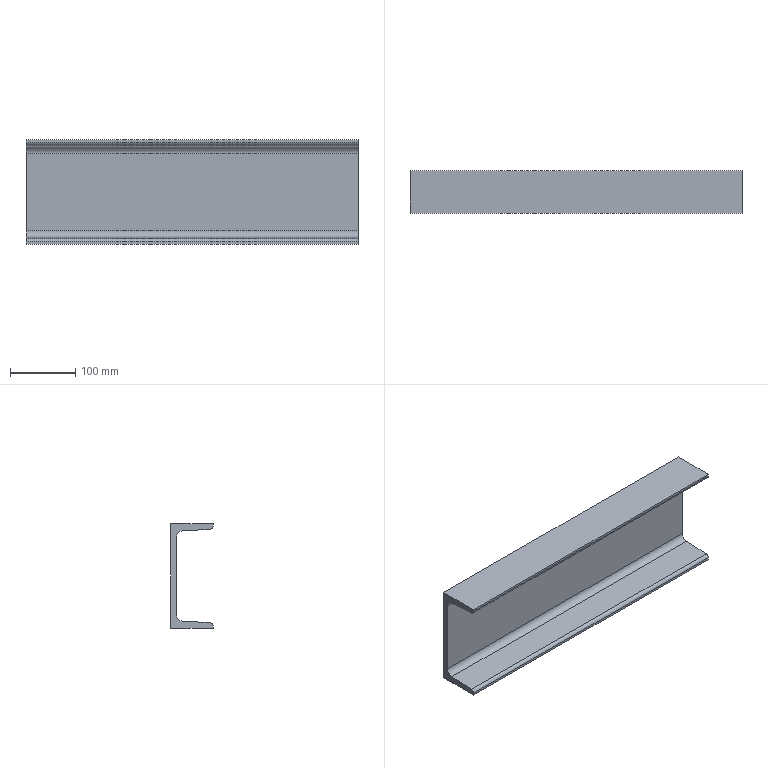Part | STEP file | 07-Channel 100x48_default<machining> | 1 solid | 14 faces | box 509 x 65 x 160 mm | volume 1267662 mm3 | plane 10 | cylinder 4 | commonest cylinder face diameters 10 x2 20 x2
STEP:
#1=CARTESIAN_POINT('',(0.,0.,0.));
#2=DIRECTION('',(0.,0.,1.));
#3=DIRECTION('',(1.,0.,0.));
#4=AXIS2_PLACEMENT_3D('',#1,#2,#3);
#5=CARTESIAN_POINT('',(0.,-65.,-160.));
#6=VERTEX_POINT('',#5);
#7=CARTESIAN_POINT('',(0.,0.,-160.));
#8=VERTEX_POINT('',#7);
#9=CARTESIAN_POINT('',(0.,0.,-160.));
#10=DIRECTION('',(0.,1.,0.));
#11=VECTOR('',#10,1.);
#12=LINE('',#9,#11);
#13=CARTESIAN_POINT('',(509.,0.,-160.));
#14=DIRECTION('',(0.,0.,1.));
#15=DIRECTION('',(1.,0.,0.));
#16=AXIS2_PLACEMENT_3D('',#13,#14,#15);
#17=PLANE('',#16);
#18=CARTESIAN_POINT('',(-509.,0.));
#19=DIRECTION('',(0.,1.));
#20=VECTOR('',#19,1.);
#21=LINE('',#18,#20);
#22=(GEOMETRIC_REPRESENTATION_CONTEXT(2)PARAMETRIC_REPRESENTATION_CONTEXT()REPRESENTATION_CONTEXT('',''));
#23=DEFINITIONAL_REPRESENTATION('',(#21),#22);
#24=PCURVE('',#17,#23);
#25=CARTESIAN_POINT('',(0.,-60.,-156.59));
#26=DIRECTION('',(1.,0.,0.));
#27=DIRECTION('',(0.,0.,-1.));
#28=AXIS2_PLACEMENT_3D('',#25,#26,#27);
#29=PLANE('',#28);
#30=CARTESIAN_POINT('',(3.41,60.));
#31=DIRECTION('',(0.,1.));
#32=VECTOR('',#31,1.);
#33=LINE('',#30,#32);
#34=(GEOMETRIC_REPRESENTATION_CONTEXT(2)PARAMETRIC_REPRESENTATION_CONTEXT()REPRESENTATION_CONTEXT('',''));
#35=DEFINITIONAL_REPRESENTATION('',(#33),#34);
#36=PCURVE('',#29,#35);
#37=SURFACE_CURVE('',#12,(#24,#36),.PCURVE_S1.);
#38=EDGE_CURVE('',#6,#8,#37,.T.);
#39=ORIENTED_EDGE('',*,*,#38,.T.);
#40=CARTESIAN_POINT('',(509.,0.,-160.));
#41=VERTEX_POINT('',#40);
#42=CARTESIAN_POINT('',(509.,0.,-160.));
#43=DIRECTION('',(-1.,0.,0.));
#44=VECTOR('',#43,1.);
#45=LINE('',#42,#44);
#46=CARTESIAN_POINT('',(0.,0.));
#47=DIRECTION('',(-1.,0.));
#48=VECTOR('',#47,1.);
#49=LINE('',#46,#48);
#50=(GEOMETRIC_REPRESENTATION_CONTEXT(2)PARAMETRIC_REPRESENTATION_CONTEXT()REPRESENTATION_CONTEXT('',''));
#51=DEFINITIONAL_REPRESENTATION('',(#49),#50);
#52=PCURVE('',#17,#51);
#53=CARTESIAN_POINT('',(509.,0.,0.));
#54=DIRECTION('',(0.,-1.,0.));
#55=DIRECTION('',(0.,0.,-1.));
#56=AXIS2_PLACEMENT_3D('',#53,#54,#55);
#57=PLANE('',#56);
#58=CARTESIAN_POINT('',(160.,0.));
#59=DIRECTION('',(0.,-1.));
#60=VECTOR('',#59,1.);
#61=LINE('',#58,#60);
#62=(GEOMETRIC_REPRESENTATION_CONTEXT(2)PARAMETRIC_REPRESENTATION_CONTEXT()REPRESENTATION_CONTEXT('',''));
#63=DEFINITIONAL_REPRESENTATION('',(#61),#62);
#64=PCURVE('',#57,#63);
#65=SURFACE_CURVE('',#45,(#52,#64),.PCURVE_S1.);
#66=EDGE_CURVE('',#41,#8,#65,.T.);
#67=ORIENTED_EDGE('',*,*,#66,.F.);
#68=CARTESIAN_POINT('',(509.,-65.,-160.));
#69=VERTEX_POINT('',#68);
#70=CARTESIAN_POINT('',(509.,0.,-160.));
#71=DIRECTION('',(0.,1.,0.));
#72=VECTOR('',#71,1.);
#73=LINE('',#70,#72);
#74=CARTESIAN_POINT('',(0.,0.));
#75=DIRECTION('',(0.,1.));
#76=VECTOR('',#75,1.);
#77=LINE('',#74,#76);
#78=(GEOMETRIC_REPRESENTATION_CONTEXT(2)PARAMETRIC_REPRESENTATION_CONTEXT()REPRESENTATION_CONTEXT('',''));
#79=DEFINITIONAL_REPRESENTATION('',(#77),#78);
#80=PCURVE('',#17,#79);
#81=CARTESIAN_POINT('',(509.,-60.,-156.59));
#82=DIRECTION('',(1.,0.,0.));
#83=DIRECTION('',(0.,0.,-1.));
#84=AXIS2_PLACEMENT_3D('',#81,#82,#83);
#85=PLANE('',#84);
#86=CARTESIAN_POINT('',(3.41,60.));
#87=DIRECTION('',(0.,1.));
#88=VECTOR('',#87,1.);
#89=LINE('',#86,#88);
#90=(GEOMETRIC_REPRESENTATION_CONTEXT(2)PARAMETRIC_REPRESENTATION_CONTEXT()REPRESENTATION_CONTEXT('',''));
#91=DEFINITIONAL_REPRESENTATION('',(#89),#90);
#92=PCURVE('',#85,#91);
#93=SURFACE_CURVE('',#73,(#80,#92),.PCURVE_S1.);
#94=EDGE_CURVE('',#69,#41,#93,.T.);
#95=ORIENTED_EDGE('',*,*,#94,.F.);
#96=CARTESIAN_POINT('',(509.,-65.,-160.));
#97=DIRECTION('',(-1.,0.,0.));
#98=VECTOR('',#97,1.);
#99=LINE('',#96,#98);
#100=CARTESIAN_POINT('',(0.,-65.));
#101=DIRECTION('',(-1.,0.));
#102=VECTOR('',#101,1.);
#103=LINE('',#100,#102);
#104=(GEOMETRIC_REPRESENTATION_CONTEXT(2)PARAMETRIC_REPRESENTATION_CONTEXT()REPRESENTATION_CONTEXT('',''));
#105=DEFINITIONAL_REPRESENTATION('',(#103),#104);
#106=PCURVE('',#17,#105);
#107=CARTESIAN_POINT('',(509.,-65.,-156.59));
#108=DIRECTION('',(0.,1.,0.));
#109=DIRECTION('',(0.,0.,1.));
#110=AXIS2_PLACEMENT_3D('',#107,#108,#109);
#111=PLANE('',#110);
#112=CARTESIAN_POINT('',(-3.41,0.));
#113=DIRECTION('',(0.,-1.));
#114=VECTOR('',#113,1.);
#115=LINE('',#112,#114);
#116=(GEOMETRIC_REPRESENTATION_CONTEXT(2)PARAMETRIC_REPRESENTATION_CONTEXT()REPRESENTATION_CONTEXT('',''));
#117=DEFINITIONAL_REPRESENTATION('',(#115),#116);
#118=PCURVE('',#111,#117);
#119=SURFACE_CURVE('',#99,(#106,#118),.PCURVE_S1.);
#120=EDGE_CURVE('',#69,#6,#119,.T.);
#121=ORIENTED_EDGE('',*,*,#120,.T.);
#122=EDGE_LOOP('',(#39,#67,#95,#121));
#123=FACE_BOUND('',#122,.T.);
#124=ADVANCED_FACE('',(#123),#17,.F.);
#125=CARTESIAN_POINT('',(0.,0.,0.));
#126=VERTEX_POINT('',#125);
#127=CARTESIAN_POINT('',(0.,0.,0.));
#128=DIRECTION('',(0.,0.,1.));
#129=VECTOR('',#128,1.);
#130=LINE('',#127,#129);
#131=CARTESIAN_POINT('',(0.,-509.));
#132=DIRECTION('',(-1.,0.));
#133=VECTOR('',#132,1.);
#134=LINE('',#131,#133);
#135=(GEOMETRIC_REPRESENTATION_CONTEXT(2)PARAMETRIC_REPRESENTATION_CONTEXT()REPRESENTATION_CONTEXT('',''));
#136=DEFINITIONAL_REPRESENTATION('',(#134),#135);
#137=PCURVE('',#57,#136);
#138=CARTESIAN_POINT('',(-156.59,60.));
#139=DIRECTION('',(-1.,0.));
#140=VECTOR('',#139,1.);
#141=LINE('',#138,#140);
#142=(GEOMETRIC_REPRESENTATION_CONTEXT(2)PARAMETRIC_REPRESENTATION_CONTEXT()REPRESENTATION_CONTEXT('',''));
#143=DEFINITIONAL_REPRESENTATION('',(#141),#142);
#144=PCURVE('',#29,#143);
#145=SURFACE_CURVE('',#130,(#137,#144),.PCURVE_S1.);
#146=EDGE_CURVE('',#8,#126,#145,.T.);
#147=ORIENTED_EDGE('',*,*,#146,.T.);
#148=CARTESIAN_POINT('',(509.,0.,0.));
#149=VERTEX_POINT('',#148);
#150=CARTESIAN_POINT('',(509.,0.,0.));
#151=DIRECTION('',(-1.,0.,0.));
#152=VECTOR('',#151,1.);
#153=LINE('',#150,#152);
#154=CARTESIAN_POINT('',(0.,0.));
#155=DIRECTION('',(0.,-1.));
#156=VECTOR('',#155,1.);
#157=LINE('',#154,#156);
#158=(GEOMETRIC_REPRESENTATION_CONTEXT(2)PARAMETRIC_REPRESENTATION_CONTEXT()REPRESENTATION_CONTEXT('',''));
#159=DEFINITIONAL_REPRESENTATION('',(#157),#158);
#160=PCURVE('',#57,#159);
#161=CARTESIAN_POINT('',(509.,0.,0.));
#162=DIRECTION('',(0.,0.,-1.));
#163=DIRECTION('',(0.,1.,0.));
#164=AXIS2_PLACEMENT_3D('',#161,#162,#163);
#165=PLANE('',#164);
#166=CARTESIAN_POINT('',(0.,0.));
#167=DIRECTION('',(0.,-1.));
#168=VECTOR('',#167,1.);
#169=LINE('',#166,#168);
#170=(GEOMETRIC_REPRESENTATION_CONTEXT(2)PARAMETRIC_REPRESENTATION_CONTEXT()REPRESENTATION_CONTEXT('',''));
#171=DEFINITIONAL_REPRESENTATION('',(#169),#170);
#172=PCURVE('',#165,#171);
#173=SURFACE_CURVE('',#153,(#160,#172),.PCURVE_S1.);
#174=EDGE_CURVE('',#149,#126,#173,.T.);
#175=ORIENTED_EDGE('',*,*,#174,.F.);
#176=CARTESIAN_POINT('',(509.,0.,0.));
#177=DIRECTION('',(0.,0.,1.));
#178=VECTOR('',#177,1.);
#179=LINE('',#176,#178);
#180=CARTESIAN_POINT('',(0.,0.));
#181=DIRECTION('',(-1.,0.));
#182=VECTOR('',#181,1.);
#183=LINE('',#180,#182);
#184=(GEOMETRIC_REPRESENTATION_CONTEXT(2)PARAMETRIC_REPRESENTATION_CONTEXT()REPRESENTATION_CONTEXT('',''));
#185=DEFINITIONAL_REPRESENTATION('',(#183),#184);
#186=PCURVE('',#57,#185);
#187=CARTESIAN_POINT('',(-156.59,60.));
#188=DIRECTION('',(-1.,0.));
#189=VECTOR('',#188,1.);
#190=LINE('',#187,#189);
#191=(GEOMETRIC_REPRESENTATION_CONTEXT(2)PARAMETRIC_REPRESENTATION_CONTEXT()REPRESENTATION_CONTEXT('',''));
#192=DEFINITIONAL_REPRESENTATION('',(#190),#191);
#193=PCURVE('',#85,#192);
#194=SURFACE_CURVE('',#179,(#186,#193),.PCURVE_S1.);
#195=EDGE_CURVE('',#41,#149,#194,.T.);
#196=ORIENTED_EDGE('',*,*,#195,.F.);
#197=ORIENTED_EDGE('',*,*,#66,.T.);
#198=EDGE_LOOP('',(#147,#175,#196,#197));
#199=FACE_BOUND('',#198,.T.);
#200=ADVANCED_FACE('',(#199),#57,.F.);
#201=CARTESIAN_POINT('',(0.,-65.,0.));
#202=VERTEX_POINT('',#201);
#203=CARTESIAN_POINT('',(0.,0.,0.));
#204=DIRECTION('',(0.,-1.,0.));
#205=VECTOR('',#204,1.);
#206=LINE('',#203,#205);
#207=CARTESIAN_POINT('',(0.,-509.));
#208=DIRECTION('',(-1.,0.));
#209=VECTOR('',#208,1.);
#210=LINE('',#207,#209);
#211=(GEOMETRIC_REPRESENTATION_CONTEXT(2)PARAMETRIC_REPRESENTATION_CONTEXT()REPRESENTATION_CONTEXT('',''));
#212=DEFINITIONAL_REPRESENTATION('',(#210),#211);
#213=PCURVE('',#165,#212);
#214=CARTESIAN_POINT('',(-156.59,60.));
#215=DIRECTION('',(0.,-1.));
#216=VECTOR('',#215,1.);
#217=LINE('',#214,#216);
#218=(GEOMETRIC_REPRESENTATION_CONTEXT(2)PARAMETRIC_REPRESENTATION_CONTEXT()REPRESENTATION_CONTEXT('',''));
#219=DEFINITIONAL_REPRESENTATION('',(#217),#218);
#220=PCURVE('',#29,#219);
#221=SURFACE_CURVE('',#206,(#213,#220),.PCURVE_S1.);
#222=EDGE_CURVE('',#126,#202,#221,.T.);
#223=ORIENTED_EDGE('',*,*,#222,.T.);
#224=CARTESIAN_POINT('',(509.,-65.,0.));
#225=VERTEX_POINT('',#224);
#226=CARTESIAN_POINT('',(509.,-65.,0.));
#227=DIRECTION('',(-1.,0.,0.));
#228=VECTOR('',#227,1.);
#229=LINE('',#226,#228);
#230=CARTESIAN_POINT('',(-65.,0.));
#231=DIRECTION('',(0.,-1.));
#232=VECTOR('',#231,1.);
#233=LINE('',#230,#232);
#234=(GEOMETRIC_REPRESENTATION_CONTEXT(2)PARAMETRIC_REPRESENTATION_CONTEXT()REPRESENTATION_CONTEXT('',''));
#235=DEFINITIONAL_REPRESENTATION('',(#233),#234);
#236=PCURVE('',#165,#235);
#237=CARTESIAN_POINT('',(509.,-65.,-3.41));
#238=DIRECTION('',(0.,1.,0.));
#239=DIRECTION('',(0.,0.,1.));
#240=AXIS2_PLACEMENT_3D('',#237,#238,#239);
#241=PLANE('',#240);
#242=CARTESIAN_POINT('',(3.41,0.));
#243=DIRECTION('',(0.,-1.));
#244=VECTOR('',#243,1.);
#245=LINE('',#242,#244);
#246=(GEOMETRIC_REPRESENTATION_CONTEXT(2)PARAMETRIC_REPRESENTATION_CONTEXT()REPRESENTATION_CONTEXT('',''));
#247=DEFINITIONAL_REPRESENTATION('',(#245),#246);
#248=PCURVE('',#241,#247);
#249=SURFACE_CURVE('',#229,(#236,#248),.PCURVE_S1.);
#250=EDGE_CURVE('',#225,#202,#249,.T.);
#251=ORIENTED_EDGE('',*,*,#250,.F.);
#252=CARTESIAN_POINT('',(509.,0.,0.));
#253=DIRECTION('',(0.,-1.,0.));
#254=VECTOR('',#253,1.);
#255=LINE('',#252,#254);
#256=CARTESIAN_POINT('',(0.,0.));
#257=DIRECTION('',(-1.,0.));
#258=VECTOR('',#257,1.);
#259=LINE('',#256,#258);
#260=(GEOMETRIC_REPRESENTATION_CONTEXT(2)PARAMETRIC_REPRESENTATION_CONTEXT()REPRESENTATION_CONTEXT('',''));
#261=DEFINITIONAL_REPRESENTATION('',(#259),#260);
#262=PCURVE('',#165,#261);
#263=CARTESIAN_POINT('',(-156.59,60.));
#264=DIRECTION('',(0.,-1.));
#265=VECTOR('',#264,1.);
#266=LINE('',#263,#265);
#267=(GEOMETRIC_REPRESENTATION_CONTEXT(2)PARAMETRIC_REPRESENTATION_CONTEXT()REPRESENTATION_CONTEXT('',''));
#268=DEFINITIONAL_REPRESENTATION('',(#266),#267);
#269=PCURVE('',#85,#268);
#270=SURFACE_CURVE('',#255,(#262,#269),.PCURVE_S1.);
#271=EDGE_CURVE('',#149,#225,#270,.T.);
#272=ORIENTED_EDGE('',*,*,#271,.F.);
#273=ORIENTED_EDGE('',*,*,#174,.T.);
#274=EDGE_LOOP('',(#223,#251,#272,#273));
#275=FACE_BOUND('',#274,.T.);
#276=ADVANCED_FACE('',(#275),#165,.F.);
#277=CARTESIAN_POINT('',(0.,-65.,-3.41));
#278=VERTEX_POINT('',#277);
#279=CARTESIAN_POINT('',(0.,-65.,-3.41));
#280=DIRECTION('',(0.,0.,-1.));
#281=VECTOR('',#280,1.);
#282=LINE('',#279,#281);
#283=CARTESIAN_POINT('',(0.,-509.));
#284=DIRECTION('',(-1.,0.));
#285=VECTOR('',#284,1.);
#286=LINE('',#283,#285);
#287=(GEOMETRIC_REPRESENTATION_CONTEXT(2)PARAMETRIC_REPRESENTATION_CONTEXT()REPRESENTATION_CONTEXT('',''));
#288=DEFINITIONAL_REPRESENTATION('',(#286),#287);
#289=PCURVE('',#241,#288);
#290=CARTESIAN_POINT('',(-153.18,-5.));
#291=DIRECTION('',(1.,0.));
#292=VECTOR('',#291,1.);
#293=LINE('',#290,#292);
#294=(GEOMETRIC_REPRESENTATION_CONTEXT(2)PARAMETRIC_REPRESENTATION_CONTEXT()REPRESENTATION_CONTEXT('',''));
#295=DEFINITIONAL_REPRESENTATION('',(#293),#294);
#296=PCURVE('',#29,#295);
#297=SURFACE_CURVE('',#282,(#289,#296),.PCURVE_S1.);
#298=EDGE_CURVE('',#202,#278,#297,.T.);
#299=ORIENTED_EDGE('',*,*,#298,.T.);
#300=CARTESIAN_POINT('',(509.,-65.,-3.41));
#301=VERTEX_POINT('',#300);
#302=CARTESIAN_POINT('',(509.,-65.,-3.41));
#303=DIRECTION('',(-1.,0.,0.));
#304=VECTOR('',#303,1.);
#305=LINE('',#302,#304);
#306=CARTESIAN_POINT('',(0.,0.));
#307=DIRECTION('',(0.,-1.));
#308=VECTOR('',#307,1.);
#309=LINE('',#306,#308);
#310=(GEOMETRIC_REPRESENTATION_CONTEXT(2)PARAMETRIC_REPRESENTATION_CONTEXT()REPRESENTATION_CONTEXT('',''));
#311=DEFINITIONAL_REPRESENTATION('',(#309),#310);
#312=PCURVE('',#241,#311);
#313=CARTESIAN_POINT('',(509.,-60.,-3.41));
#314=DIRECTION('',(-1.,0.,0.));
#315=DIRECTION('',(0.,0.,1.));
#316=AXIS2_PLACEMENT_3D('',#313,#314,#315);
#317=CYLINDRICAL_SURFACE('',#316,5.);
#318=CARTESIAN_POINT('',(4.712,0.));
#319=DIRECTION('',(0.,1.));
#320=VECTOR('',#319,1.);
#321=LINE('',#318,#320);
#322=(GEOMETRIC_REPRESENTATION_CONTEXT(2)PARAMETRIC_REPRESENTATION_CONTEXT()REPRESENTATION_CONTEXT('',''));
#323=DEFINITIONAL_REPRESENTATION('',(#321),#322);
#324=PCURVE('',#317,#323);
#325=SURFACE_CURVE('',#305,(#312,#324),.PCURVE_S1.);
#326=EDGE_CURVE('',#301,#278,#325,.T.);
#327=ORIENTED_EDGE('',*,*,#326,.F.);
#328=CARTESIAN_POINT('',(509.,-65.,-3.41));
#329=DIRECTION('',(0.,0.,-1.));
#330=VECTOR('',#329,1.);
#331=LINE('',#328,#330);
#332=CARTESIAN_POINT('',(0.,0.));
#333=DIRECTION('',(-1.,0.));
#334=VECTOR('',#333,1.);
#335=LINE('',#332,#334);
#336=(GEOMETRIC_REPRESENTATION_CONTEXT(2)PARAMETRIC_REPRESENTATION_CONTEXT()REPRESENTATION_CONTEXT('',''));
#337=DEFINITIONAL_REPRESENTATION('',(#335),#336);
#338=PCURVE('',#241,#337);
#339=CARTESIAN_POINT('',(-153.18,-5.));
#340=DIRECTION('',(1.,0.));
#341=VECTOR('',#340,1.);
#342=LINE('',#339,#341);
#343=(GEOMETRIC_REPRESENTATION_CONTEXT(2)PARAMETRIC_REPRESENTATION_CONTEXT()REPRESENTATION_CONTEXT('',''));
#344=DEFINITIONAL_REPRESENTATION('',(#342),#343);
#345=PCURVE('',#85,#344);
#346=SURFACE_CURVE('',#331,(#338,#345),.PCURVE_S1.);
#347=EDGE_CURVE('',#225,#301,#346,.T.);
#348=ORIENTED_EDGE('',*,*,#347,.F.);
#349=ORIENTED_EDGE('',*,*,#250,.T.);
#350=EDGE_LOOP('',(#299,#327,#348,#349));
#351=FACE_BOUND('',#350,.T.);
#352=ADVANCED_FACE('',(#351),#241,.F.);
#353=CARTESIAN_POINT('',(0.,-60.287,-8.402));
#354=VERTEX_POINT('',#353);
#355=CARTESIAN_POINT('',(0.,-60.,-3.41));
#356=DIRECTION('',(1.,0.,0.));
#357=DIRECTION('',(0.,0.,-1.));
#358=AXIS2_PLACEMENT_3D('',#355,#356,#357);
#359=CIRCLE('',#358,5.);
#360=CARTESIAN_POINT('',(9.425,509.));
#361=DIRECTION('',(-1.,0.));
#362=VECTOR('',#361,1.);
#363=LINE('',#360,#362);
#364=(GEOMETRIC_REPRESENTATION_CONTEXT(2)PARAMETRIC_REPRESENTATION_CONTEXT()REPRESENTATION_CONTEXT('',''));
#365=DEFINITIONAL_REPRESENTATION('',(#363),#364);
#366=PCURVE('',#317,#365);
#367=CARTESIAN_POINT('',(-153.18,0.));
#368=DIRECTION('',(1.,0.));
#369=AXIS2_PLACEMENT_2D('',#367,#368);
#370=CIRCLE('',#369,5.);
#371=(GEOMETRIC_REPRESENTATION_CONTEXT(2)PARAMETRIC_REPRESENTATION_CONTEXT()REPRESENTATION_CONTEXT('',''));
#372=DEFINITIONAL_REPRESENTATION('',(#370),#371);
#373=PCURVE('',#29,#372);
#374=SURFACE_CURVE('',#359,(#366,#373),.PCURVE_S1.);
#375=EDGE_CURVE('',#278,#354,#374,.T.);
#376=ORIENTED_EDGE('',*,*,#375,.T.);
#377=CARTESIAN_POINT('',(509.,-60.287,-8.402));
#378=VERTEX_POINT('',#377);
#379=CARTESIAN_POINT('',(509.,-60.287,-8.402));
#380=DIRECTION('',(-1.,0.,0.));
#381=VECTOR('',#380,1.);
#382=LINE('',#379,#381);
#383=CARTESIAN_POINT('',(3.199,0.));
#384=DIRECTION('',(0.,1.));
#385=VECTOR('',#384,1.);
#386=LINE('',#383,#385);
#387=(GEOMETRIC_REPRESENTATION_CONTEXT(2)PARAMETRIC_REPRESENTATION_CONTEXT()REPRESENTATION_CONTEXT('',''));
#388=DEFINITIONAL_REPRESENTATION('',(#386),#387);
#389=PCURVE('',#317,#388);
#390=CARTESIAN_POINT('',(509.,-17.926,-10.838));
#391=DIRECTION('',(0.,0.05743,0.9983));
#392=DIRECTION('',(0.,-0.9983,0.05743));
#393=AXIS2_PLACEMENT_3D('',#390,#391,#392);
#394=PLANE('',#393);
#395=CARTESIAN_POINT('',(42.431,0.));
#396=DIRECTION('',(0.,-1.));
#397=VECTOR('',#396,1.);
#398=LINE('',#395,#397);
#399=(GEOMETRIC_REPRESENTATION_CONTEXT(2)PARAMETRIC_REPRESENTATION_CONTEXT()REPRESENTATION_CONTEXT('',''));
#400=DEFINITIONAL_REPRESENTATION('',(#398),#399);
#401=PCURVE('',#394,#400);
#402=SURFACE_CURVE('',#382,(#389,#401),.PCURVE_S1.);
#403=EDGE_CURVE('',#378,#354,#402,.T.);
#404=ORIENTED_EDGE('',*,*,#403,.F.);
#405=CARTESIAN_POINT('',(509.,-60.,-3.41));
#406=DIRECTION('',(1.,0.,0.));
#407=DIRECTION('',(0.,0.,-1.));
#408=AXIS2_PLACEMENT_3D('',#405,#406,#407);
#409=CIRCLE('',#408,5.);
#410=CARTESIAN_POINT('',(9.425,0.));
#411=DIRECTION('',(-1.,0.));
#412=VECTOR('',#411,1.);
#413=LINE('',#410,#412);
#414=(GEOMETRIC_REPRESENTATION_CONTEXT(2)PARAMETRIC_REPRESENTATION_CONTEXT()REPRESENTATION_CONTEXT('',''));
#415=DEFINITIONAL_REPRESENTATION('',(#413),#414);
#416=PCURVE('',#317,#415);
#417=CARTESIAN_POINT('',(-153.18,0.));
#418=DIRECTION('',(1.,0.));
#419=AXIS2_PLACEMENT_2D('',#417,#418);
#420=CIRCLE('',#419,5.);
#421=(GEOMETRIC_REPRESENTATION_CONTEXT(2)PARAMETRIC_REPRESENTATION_CONTEXT()REPRESENTATION_CONTEXT('',''));
#422=DEFINITIONAL_REPRESENTATION('',(#420),#421);
#423=PCURVE('',#85,#422);
#424=SURFACE_CURVE('',#409,(#416,#423),.PCURVE_S1.);
#425=EDGE_CURVE('',#301,#378,#424,.T.);
#426=ORIENTED_EDGE('',*,*,#425,.F.);
#427=ORIENTED_EDGE('',*,*,#326,.T.);
#428=EDGE_LOOP('',(#376,#404,#426,#427));
#429=FACE_BOUND('',#428,.T.);
#430=ADVANCED_FACE('',(#429),#317,.T.);
#431=CARTESIAN_POINT('',(0.,-17.926,-10.838));
#432=VERTEX_POINT('',#431);
#433=CARTESIAN_POINT('',(0.,-17.926,-10.838));
#434=DIRECTION('',(0.,0.9983,-0.05743));
#435=VECTOR('',#434,1.);
#436=LINE('',#433,#435);
#437=CARTESIAN_POINT('',(0.,-509.));
#438=DIRECTION('',(-1.,0.));
#439=VECTOR('',#438,1.);
#440=LINE('',#437,#439);
#441=(GEOMETRIC_REPRESENTATION_CONTEXT(2)PARAMETRIC_REPRESENTATION_CONTEXT()REPRESENTATION_CONTEXT('',''));
#442=DEFINITIONAL_REPRESENTATION('',(#440),#441);
#443=PCURVE('',#394,#442);
#444=CARTESIAN_POINT('',(-145.752,42.074));
#445=DIRECTION('',(0.05743,0.9983));
#446=VECTOR('',#445,1.);
#447=LINE('',#444,#446);
#448=(GEOMETRIC_REPRESENTATION_CONTEXT(2)PARAMETRIC_REPRESENTATION_CONTEXT()REPRESENTATION_CONTEXT('',''));
#449=DEFINITIONAL_REPRESENTATION('',(#447),#448);
#450=PCURVE('',#29,#449);
#451=SURFACE_CURVE('',#436,(#443,#450),.PCURVE_S1.);
#452=EDGE_CURVE('',#354,#432,#451,.T.);
#453=ORIENTED_EDGE('',*,*,#452,.T.);
#454=CARTESIAN_POINT('',(509.,-17.926,-10.838));
#455=VERTEX_POINT('',#454);
#456=CARTESIAN_POINT('',(509.,-17.926,-10.838));
#457=DIRECTION('',(-1.,0.,0.));
#458=VECTOR('',#457,1.);
#459=LINE('',#456,#458);
#460=CARTESIAN_POINT('',(0.,0.));
#461=DIRECTION('',(0.,-1.));
#462=VECTOR('',#461,1.);
#463=LINE('',#460,#462);
#464=(GEOMETRIC_REPRESENTATION_CONTEXT(2)PARAMETRIC_REPRESENTATION_CONTEXT()REPRESENTATION_CONTEXT('',''));
#465=DEFINITIONAL_REPRESENTATION('',(#463),#464);
#466=PCURVE('',#394,#465);
#467=CARTESIAN_POINT('',(509.,-18.5,-20.822));
#468=DIRECTION('',(-1.,0.,0.));
#469=DIRECTION('',(0.,0.,1.));
#470=AXIS2_PLACEMENT_3D('',#467,#468,#469);
#471=CYLINDRICAL_SURFACE('',#470,10.);
#472=CARTESIAN_POINT('',(0.05746,0.));
#473=DIRECTION('',(0.,1.));
#474=VECTOR('',#473,1.);
#475=LINE('',#472,#474);
#476=(GEOMETRIC_REPRESENTATION_CONTEXT(2)PARAMETRIC_REPRESENTATION_CONTEXT()REPRESENTATION_CONTEXT('',''));
#477=DEFINITIONAL_REPRESENTATION('',(#475),#476);
#478=PCURVE('',#471,#477);
#479=SURFACE_CURVE('',#459,(#466,#478),.PCURVE_S1.);
#480=EDGE_CURVE('',#455,#432,#479,.T.);
#481=ORIENTED_EDGE('',*,*,#480,.F.);
#482=CARTESIAN_POINT('',(509.,-17.926,-10.838));
#483=DIRECTION('',(0.,0.9983,-0.05743));
#484=VECTOR('',#483,1.);
#485=LINE('',#482,#484);
#486=CARTESIAN_POINT('',(0.,0.));
#487=DIRECTION('',(-1.,0.));
#488=VECTOR('',#487,1.);
#489=LINE('',#486,#488);
#490=(GEOMETRIC_REPRESENTATION_CONTEXT(2)PARAMETRIC_REPRESENTATION_CONTEXT()REPRESENTATION_CONTEXT('',''));
#491=DEFINITIONAL_REPRESENTATION('',(#489),#490);
#492=PCURVE('',#394,#491);
#493=CARTESIAN_POINT('',(-145.752,42.074));
#494=DIRECTION('',(0.05743,0.9983));
#495=VECTOR('',#494,1.);
#496=LINE('',#493,#495);
#497=(GEOMETRIC_REPRESENTATION_CONTEXT(2)PARAMETRIC_REPRESENTATION_CONTEXT()REPRESENTATION_CONTEXT('',''));
#498=DEFINITIONAL_REPRESENTATION('',(#496),#497);
#499=PCURVE('',#85,#498);
#500=SURFACE_CURVE('',#485,(#492,#499),.PCURVE_S1.);
#501=EDGE_CURVE('',#378,#455,#500,.T.);
#502=ORIENTED_EDGE('',*,*,#501,.F.);
#503=ORIENTED_EDGE('',*,*,#403,.T.);
#504=EDGE_LOOP('',(#453,#481,#502,#503));
#505=FACE_BOUND('',#504,.T.);
#506=ADVANCED_FACE('',(#505),#394,.F.);
#507=ORIENTED_EDGE('',*,*,#480,.F.);
#508=CARTESIAN_POINT('',(509.,-8.5,-20.822));
#509=VERTEX_POINT('',#508);
#510=CARTESIAN_POINT('',(509.,-18.5,-20.822));
#511=DIRECTION('',(-1.,0.,0.));
#512=DIRECTION('',(0.,0.,1.));
#513=AXIS2_PLACEMENT_3D('',#510,#511,#512);
#514=CIRCLE('',#513,10.);
#515=CARTESIAN_POINT('',(0.,0.));
#516=DIRECTION('',(1.,0.));
#517=VECTOR('',#516,1.);
#518=LINE('',#515,#517);
#519=(GEOMETRIC_REPRESENTATION_CONTEXT(2)PARAMETRIC_REPRESENTATION_CONTEXT()REPRESENTATION_CONTEXT('',''));
#520=DEFINITIONAL_REPRESENTATION('',(#518),#519);
#521=PCURVE('',#471,#520);
#522=CARTESIAN_POINT('',(-145.768,41.5));
#523=CARTESIAN_POINT('',(-145.768,58.821));
#524=CARTESIAN_POINT('',(-130.768,50.16));
#525=CARTESIAN_POINT('',(-115.768,41.5));
#526=CARTESIAN_POINT('',(-130.768,32.84));
#527=CARTESIAN_POINT('',(-145.768,24.179));
#528=CARTESIAN_POINT('',(-145.768,41.5));
#529=(BOUNDED_CURVE()B_SPLINE_CURVE(2,(#522,#523,#524,#525,#526,#527,#528),.UNSPECIFIED.,.T.,.F.)B_SPLINE_CURVE_WITH_KNOTS((1,2,2,2,2,1),(-2.094,0.,2.094,4.189,6.283,8.378),.UNSPECIFIED.)CURVE()GEOMETRIC_REPRESENTATION_ITEM()RATIONAL_B_SPLINE_CURVE((1.,0.5,1.,0.5,1.,0.5,1.))REPRESENTATION_ITEM(''));
#530=(GEOMETRIC_REPRESENTATION_CONTEXT(2)PARAMETRIC_REPRESENTATION_CONTEXT()REPRESENTATION_CONTEXT('',''));
#531=DEFINITIONAL_REPRESENTATION('',(#529),#530);
#532=PCURVE('',#85,#531);
#533=SURFACE_CURVE('',#514,(#521,#532),.PCURVE_S1.);
#534=EDGE_CURVE('',#455,#509,#533,.T.);
#535=ORIENTED_EDGE('',*,*,#534,.T.);
#536=CARTESIAN_POINT('',(0.,-8.5,-20.822));
#537=VERTEX_POINT('',#536);
#538=CARTESIAN_POINT('',(509.,-8.5,-20.822));
#539=DIRECTION('',(-1.,0.,0.));
#540=VECTOR('',#539,1.);
#541=LINE('',#538,#540);
#542=CARTESIAN_POINT('',(1.571,0.));
#543=DIRECTION('',(0.,1.));
#544=VECTOR('',#543,1.);
#545=LINE('',#542,#544);
#546=(GEOMETRIC_REPRESENTATION_CONTEXT(2)PARAMETRIC_REPRESENTATION_CONTEXT()REPRESENTATION_CONTEXT('',''));
#547=DEFINITIONAL_REPRESENTATION('',(#545),#546);
#548=PCURVE('',#471,#547);
#549=CARTESIAN_POINT('',(509.,-8.5,-139.178));
#550=DIRECTION('',(0.,1.,0.));
#551=DIRECTION('',(0.,0.,1.));
#552=AXIS2_PLACEMENT_3D('',#549,#550,#551);
#553=PLANE('',#552);
#554=CARTESIAN_POINT('',(118.356,0.));
#555=DIRECTION('',(0.,-1.));
#556=VECTOR('',#555,1.);
#557=LINE('',#554,#556);
#558=(GEOMETRIC_REPRESENTATION_CONTEXT(2)PARAMETRIC_REPRESENTATION_CONTEXT()REPRESENTATION_CONTEXT('',''));
#559=DEFINITIONAL_REPRESENTATION('',(#557),#558);
#560=PCURVE('',#553,#559);
#561=SURFACE_CURVE('',#541,(#548,#560),.PCURVE_S1.);
#562=EDGE_CURVE('',#509,#537,#561,.T.);
#563=ORIENTED_EDGE('',*,*,#562,.T.);
#564=CARTESIAN_POINT('',(0.,-18.5,-20.822));
#565=DIRECTION('',(-1.,0.,0.));
#566=DIRECTION('',(0.,0.,1.));
#567=AXIS2_PLACEMENT_3D('',#564,#565,#566);
#568=CIRCLE('',#567,10.);
#569=CARTESIAN_POINT('',(0.,509.));
#570=DIRECTION('',(1.,0.));
#571=VECTOR('',#570,1.);
#572=LINE('',#569,#571);
#573=(GEOMETRIC_REPRESENTATION_CONTEXT(2)PARAMETRIC_REPRESENTATION_CONTEXT()REPRESENTATION_CONTEXT('',''));
#574=DEFINITIONAL_REPRESENTATION('',(#572),#573);
#575=PCURVE('',#471,#574);
#576=CARTESIAN_POINT('',(-145.768,41.5));
#577=CARTESIAN_POINT('',(-145.768,58.821));
#578=CARTESIAN_POINT('',(-130.768,50.16));
#579=CARTESIAN_POINT('',(-115.768,41.5));
#580=CARTESIAN_POINT('',(-130.768,32.84));
#581=CARTESIAN_POINT('',(-145.768,24.179));
#582=CARTESIAN_POINT('',(-145.768,41.5));
#583=(BOUNDED_CURVE()B_SPLINE_CURVE(2,(#576,#577,#578,#579,#580,#581,#582),.UNSPECIFIED.,.T.,.F.)B_SPLINE_CURVE_WITH_KNOTS((1,2,2,2,2,1),(-2.094,0.,2.094,4.189,6.283,8.378),.UNSPECIFIED.)CURVE()GEOMETRIC_REPRESENTATION_ITEM()RATIONAL_B_SPLINE_CURVE((1.,0.5,1.,0.5,1.,0.5,1.))REPRESENTATION_ITEM(''));
#584=(GEOMETRIC_REPRESENTATION_CONTEXT(2)PARAMETRIC_REPRESENTATION_CONTEXT()REPRESENTATION_CONTEXT('',''));
#585=DEFINITIONAL_REPRESENTATION('',(#583),#584);
#586=PCURVE('',#29,#585);
#587=SURFACE_CURVE('',#568,(#575,#586),.PCURVE_S1.);
#588=EDGE_CURVE('',#432,#537,#587,.T.);
#589=ORIENTED_EDGE('',*,*,#588,.F.);
#590=EDGE_LOOP('',(#507,#535,#563,#589));
#591=FACE_BOUND('',#590,.F.);
#592=ADVANCED_FACE('',(#591),#471,.F.);
#593=CARTESIAN_POINT('',(0.,-8.5,-139.178));
#594=VERTEX_POINT('',#593);
#595=CARTESIAN_POINT('',(0.,-8.5,-139.178));
#596=DIRECTION('',(0.,0.,-1.));
#597=VECTOR('',#596,1.);
#598=LINE('',#595,#597);
#599=CARTESIAN_POINT('',(0.,-509.));
#600=DIRECTION('',(-1.,0.));
#601=VECTOR('',#600,1.);
#602=LINE('',#599,#601);
#603=(GEOMETRIC_REPRESENTATION_CONTEXT(2)PARAMETRIC_REPRESENTATION_CONTEXT()REPRESENTATION_CONTEXT('',''));
#604=DEFINITIONAL_REPRESENTATION('',(#602),#603);
#605=PCURVE('',#553,#604);
#606=CARTESIAN_POINT('',(-17.412,51.5));
#607=DIRECTION('',(1.,0.));
#608=VECTOR('',#607,1.);
#609=LINE('',#606,#608);
#610=(GEOMETRIC_REPRESENTATION_CONTEXT(2)PARAMETRIC_REPRESENTATION_CONTEXT()REPRESENTATION_CONTEXT('',''));
#611=DEFINITIONAL_REPRESENTATION('',(#609),#610);
#612=PCURVE('',#29,#611);
#613=SURFACE_CURVE('',#598,(#605,#612),.PCURVE_S1.);
#614=EDGE_CURVE('',#537,#594,#613,.T.);
#615=ORIENTED_EDGE('',*,*,#614,.T.);
#616=CARTESIAN_POINT('',(509.,-8.5,-139.178));
#617=VERTEX_POINT('',#616);
#618=CARTESIAN_POINT('',(509.,-8.5,-139.178));
#619=DIRECTION('',(-1.,0.,0.));
#620=VECTOR('',#619,1.);
#621=LINE('',#618,#620);
#622=CARTESIAN_POINT('',(0.,0.));
#623=DIRECTION('',(0.,-1.));
#624=VECTOR('',#623,1.);
#625=LINE('',#622,#624);
#626=(GEOMETRIC_REPRESENTATION_CONTEXT(2)PARAMETRIC_REPRESENTATION_CONTEXT()REPRESENTATION_CONTEXT('',''));
#627=DEFINITIONAL_REPRESENTATION('',(#625),#626);
#628=PCURVE('',#553,#627);
#629=CARTESIAN_POINT('',(509.,-18.5,-139.178));
#630=DIRECTION('',(-1.,0.,0.));
#631=DIRECTION('',(0.,0.,1.));
#632=AXIS2_PLACEMENT_3D('',#629,#630,#631);
#633=CYLINDRICAL_SURFACE('',#632,10.);
#634=CARTESIAN_POINT('',(1.571,0.));
#635=DIRECTION('',(0.,1.));
#636=VECTOR('',#635,1.);
#637=LINE('',#634,#636);
#638=(GEOMETRIC_REPRESENTATION_CONTEXT(2)PARAMETRIC_REPRESENTATION_CONTEXT()REPRESENTATION_CONTEXT('',''));
#639=DEFINITIONAL_REPRESENTATION('',(#637),#638);
#640=PCURVE('',#633,#639);
#641=SURFACE_CURVE('',#621,(#628,#640),.PCURVE_S1.);
#642=EDGE_CURVE('',#617,#594,#641,.T.);
#643=ORIENTED_EDGE('',*,*,#642,.F.);
#644=CARTESIAN_POINT('',(509.,-8.5,-139.178));
#645=DIRECTION('',(0.,0.,-1.));
#646=VECTOR('',#645,1.);
#647=LINE('',#644,#646);
#648=CARTESIAN_POINT('',(0.,0.));
#649=DIRECTION('',(-1.,0.));
#650=VECTOR('',#649,1.);
#651=LINE('',#648,#650);
#652=(GEOMETRIC_REPRESENTATION_CONTEXT(2)PARAMETRIC_REPRESENTATION_CONTEXT()REPRESENTATION_CONTEXT('',''));
#653=DEFINITIONAL_REPRESENTATION('',(#651),#652);
#654=PCURVE('',#553,#653);
#655=CARTESIAN_POINT('',(-17.412,51.5));
#656=DIRECTION('',(1.,0.));
#657=VECTOR('',#656,1.);
#658=LINE('',#655,#657);
#659=(GEOMETRIC_REPRESENTATION_CONTEXT(2)PARAMETRIC_REPRESENTATION_CONTEXT()REPRESENTATION_CONTEXT('',''));
#660=DEFINITIONAL_REPRESENTATION('',(#658),#659);
#661=PCURVE('',#85,#660);
#662=SURFACE_CURVE('',#647,(#654,#661),.PCURVE_S1.);
#663=EDGE_CURVE('',#509,#617,#662,.T.);
#664=ORIENTED_EDGE('',*,*,#663,.F.);
#665=ORIENTED_EDGE('',*,*,#562,.T.);
#666=EDGE_LOOP('',(#615,#643,#664,#665));
#667=FACE_BOUND('',#666,.T.);
#668=ADVANCED_FACE('',(#667),#553,.F.);
#669=ORIENTED_EDGE('',*,*,#642,.F.);
#670=CARTESIAN_POINT('',(509.,-17.926,-149.162));
#671=VERTEX_POINT('',#670);
#672=CARTESIAN_POINT('',(509.,-18.5,-139.178));
#673=DIRECTION('',(-1.,0.,0.));
#674=DIRECTION('',(0.,0.,1.));
#675=AXIS2_PLACEMENT_3D('',#672,#673,#674);
#676=CIRCLE('',#675,10.);
#677=CARTESIAN_POINT('',(0.,0.));
#678=DIRECTION('',(1.,0.));
#679=VECTOR('',#678,1.);
#680=LINE('',#677,#679);
#681=(GEOMETRIC_REPRESENTATION_CONTEXT(2)PARAMETRIC_REPRESENTATION_CONTEXT()REPRESENTATION_CONTEXT('',''));
#682=DEFINITIONAL_REPRESENTATION('',(#680),#681);
#683=PCURVE('',#633,#682);
#684=CARTESIAN_POINT('',(-27.412,41.5));
#685=CARTESIAN_POINT('',(-27.412,58.821));
#686=CARTESIAN_POINT('',(-12.412,50.16));
#687=CARTESIAN_POINT('',(2.588,41.5));
#688=CARTESIAN_POINT('',(-12.412,32.84));
#689=CARTESIAN_POINT('',(-27.412,24.179));
#690=CARTESIAN_POINT('',(-27.412,41.5));
#691=(BOUNDED_CURVE()B_SPLINE_CURVE(2,(#684,#685,#686,#687,#688,#689,#690),.UNSPECIFIED.,.T.,.F.)B_SPLINE_CURVE_WITH_KNOTS((1,2,2,2,2,1),(-2.094,0.,2.094,4.189,6.283,8.378),.UNSPECIFIED.)CURVE()GEOMETRIC_REPRESENTATION_ITEM()RATIONAL_B_SPLINE_CURVE((1.,0.5,1.,0.5,1.,0.5,1.))REPRESENTATION_ITEM(''));
#692=(GEOMETRIC_REPRESENTATION_CONTEXT(2)PARAMETRIC_REPRESENTATION_CONTEXT()REPRESENTATION_CONTEXT('',''));
#693=DEFINITIONAL_REPRESENTATION('',(#691),#692);
#694=PCURVE('',#85,#693);
#695=SURFACE_CURVE('',#676,(#683,#694),.PCURVE_S1.);
#696=EDGE_CURVE('',#617,#671,#695,.T.);
#697=ORIENTED_EDGE('',*,*,#696,.T.);
#698=CARTESIAN_POINT('',(0.,-17.926,-149.162));
#699=VERTEX_POINT('',#698);
#700=CARTESIAN_POINT('',(509.,-17.926,-149.162));
#701=DIRECTION('',(-1.,0.,0.));
#702=VECTOR('',#701,1.);
#703=LINE('',#700,#702);
#704=CARTESIAN_POINT('',(3.084,0.));
#705=DIRECTION('',(0.,1.));
#706=VECTOR('',#705,1.);
#707=LINE('',#704,#706);
#708=(GEOMETRIC_REPRESENTATION_CONTEXT(2)PARAMETRIC_REPRESENTATION_CONTEXT()REPRESENTATION_CONTEXT('',''));
#709=DEFINITIONAL_REPRESENTATION('',(#707),#708);
#710=PCURVE('',#633,#709);
#711=CARTESIAN_POINT('',(509.,-17.926,-149.162));
#712=DIRECTION('',(0.,0.05743,-0.9983));
#713=DIRECTION('',(0.,0.9983,0.05743));
#714=AXIS2_PLACEMENT_3D('',#711,#712,#713);
#715=PLANE('',#714);
#716=CARTESIAN_POINT('',(0.,0.));
#717=DIRECTION('',(0.,-1.));
#718=VECTOR('',#717,1.);
#719=LINE('',#716,#718);
#720=(GEOMETRIC_REPRESENTATION_CONTEXT(2)PARAMETRIC_REPRESENTATION_CONTEXT()REPRESENTATION_CONTEXT('',''));
#721=DEFINITIONAL_REPRESENTATION('',(#719),#720);
#722=PCURVE('',#715,#721);
#723=SURFACE_CURVE('',#703,(#710,#722),.PCURVE_S1.);
#724=EDGE_CURVE('',#671,#699,#723,.T.);
#725=ORIENTED_EDGE('',*,*,#724,.T.);
#726=CARTESIAN_POINT('',(0.,-18.5,-139.178));
#727=DIRECTION('',(-1.,0.,0.));
#728=DIRECTION('',(0.,0.,1.));
#729=AXIS2_PLACEMENT_3D('',#726,#727,#728);
#730=CIRCLE('',#729,10.);
#731=CARTESIAN_POINT('',(0.,509.));
#732=DIRECTION('',(1.,0.));
#733=VECTOR('',#732,1.);
#734=LINE('',#731,#733);
#735=(GEOMETRIC_REPRESENTATION_CONTEXT(2)PARAMETRIC_REPRESENTATION_CONTEXT()REPRESENTATION_CONTEXT('',''));
#736=DEFINITIONAL_REPRESENTATION('',(#734),#735);
#737=PCURVE('',#633,#736);
#738=CARTESIAN_POINT('',(-27.412,41.5));
#739=CARTESIAN_POINT('',(-27.412,58.821));
#740=CARTESIAN_POINT('',(-12.412,50.16));
#741=CARTESIAN_POINT('',(2.588,41.5));
#742=CARTESIAN_POINT('',(-12.412,32.84));
#743=CARTESIAN_POINT('',(-27.412,24.179));
#744=CARTESIAN_POINT('',(-27.412,41.5));
#745=(BOUNDED_CURVE()B_SPLINE_CURVE(2,(#738,#739,#740,#741,#742,#743,#744),.UNSPECIFIED.,.T.,.F.)B_SPLINE_CURVE_WITH_KNOTS((1,2,2,2,2,1),(-2.094,0.,2.094,4.189,6.283,8.378),.UNSPECIFIED.)CURVE()GEOMETRIC_REPRESENTATION_ITEM()RATIONAL_B_SPLINE_CURVE((1.,0.5,1.,0.5,1.,0.5,1.))REPRESENTATION_ITEM(''));
#746=(GEOMETRIC_REPRESENTATION_CONTEXT(2)PARAMETRIC_REPRESENTATION_CONTEXT()REPRESENTATION_CONTEXT('',''));
#747=DEFINITIONAL_REPRESENTATION('',(#745),#746);
#748=PCURVE('',#29,#747);
#749=SURFACE_CURVE('',#730,(#737,#748),.PCURVE_S1.);
#750=EDGE_CURVE('',#594,#699,#749,.T.);
#751=ORIENTED_EDGE('',*,*,#750,.F.);
#752=EDGE_LOOP('',(#669,#697,#725,#751));
#753=FACE_BOUND('',#752,.F.);
#754=ADVANCED_FACE('',(#753),#633,.F.);
#755=CARTESIAN_POINT('',(0.,-60.287,-151.598));
#756=VERTEX_POINT('',#755);
#757=CARTESIAN_POINT('',(0.,-17.926,-149.162));
#758=DIRECTION('',(0.,-0.9983,-0.05743));
#759=VECTOR('',#758,1.);
#760=LINE('',#757,#759);
#761=CARTESIAN_POINT('',(0.,-509.));
#762=DIRECTION('',(-1.,0.));
#763=VECTOR('',#762,1.);
#764=LINE('',#761,#763);
#765=(GEOMETRIC_REPRESENTATION_CONTEXT(2)PARAMETRIC_REPRESENTATION_CONTEXT()REPRESENTATION_CONTEXT('',''));
#766=DEFINITIONAL_REPRESENTATION('',(#764),#765);
#767=PCURVE('',#715,#766);
#768=CARTESIAN_POINT('',(-7.428,42.074));
#769=DIRECTION('',(0.05743,-0.9983));
#770=VECTOR('',#769,1.);
#771=LINE('',#768,#770);
#772=(GEOMETRIC_REPRESENTATION_CONTEXT(2)PARAMETRIC_REPRESENTATION_CONTEXT()REPRESENTATION_CONTEXT('',''));
#773=DEFINITIONAL_REPRESENTATION('',(#771),#772);
#774=PCURVE('',#29,#773);
#775=SURFACE_CURVE('',#760,(#767,#774),.PCURVE_S1.);
#776=EDGE_CURVE('',#699,#756,#775,.T.);
#777=ORIENTED_EDGE('',*,*,#776,.T.);
#778=CARTESIAN_POINT('',(509.,-60.287,-151.598));
#779=VERTEX_POINT('',#778);
#780=CARTESIAN_POINT('',(509.,-60.287,-151.598));
#781=DIRECTION('',(-1.,0.,0.));
#782=VECTOR('',#781,1.);
#783=LINE('',#780,#782);
#784=CARTESIAN_POINT('',(-42.431,0.));
#785=DIRECTION('',(0.,-1.));
#786=VECTOR('',#785,1.);
#787=LINE('',#784,#786);
#788=(GEOMETRIC_REPRESENTATION_CONTEXT(2)PARAMETRIC_REPRESENTATION_CONTEXT()REPRESENTATION_CONTEXT('',''));
#789=DEFINITIONAL_REPRESENTATION('',(#787),#788);
#790=PCURVE('',#715,#789);
#791=CARTESIAN_POINT('',(509.,-60.,-156.59));
#792=DIRECTION('',(-1.,0.,0.));
#793=DIRECTION('',(0.,0.,1.));
#794=AXIS2_PLACEMENT_3D('',#791,#792,#793);
#795=CYLINDRICAL_SURFACE('',#794,5.);
#796=CARTESIAN_POINT('',(6.226,0.));
#797=DIRECTION('',(0.,1.));
#798=VECTOR('',#797,1.);
#799=LINE('',#796,#798);
#800=(GEOMETRIC_REPRESENTATION_CONTEXT(2)PARAMETRIC_REPRESENTATION_CONTEXT()REPRESENTATION_CONTEXT('',''));
#801=DEFINITIONAL_REPRESENTATION('',(#799),#800);
#802=PCURVE('',#795,#801);
#803=SURFACE_CURVE('',#783,(#790,#802),.PCURVE_S1.);
#804=EDGE_CURVE('',#779,#756,#803,.T.);
#805=ORIENTED_EDGE('',*,*,#804,.F.);
#806=CARTESIAN_POINT('',(509.,-17.926,-149.162));
#807=DIRECTION('',(0.,-0.9983,-0.05743));
#808=VECTOR('',#807,1.);
#809=LINE('',#806,#808);
#810=CARTESIAN_POINT('',(0.,0.));
#811=DIRECTION('',(-1.,0.));
#812=VECTOR('',#811,1.);
#813=LINE('',#810,#812);
#814=(GEOMETRIC_REPRESENTATION_CONTEXT(2)PARAMETRIC_REPRESENTATION_CONTEXT()REPRESENTATION_CONTEXT('',''));
#815=DEFINITIONAL_REPRESENTATION('',(#813),#814);
#816=PCURVE('',#715,#815);
#817=CARTESIAN_POINT('',(-7.428,42.074));
#818=DIRECTION('',(0.05743,-0.9983));
#819=VECTOR('',#818,1.);
#820=LINE('',#817,#819);
#821=(GEOMETRIC_REPRESENTATION_CONTEXT(2)PARAMETRIC_REPRESENTATION_CONTEXT()REPRESENTATION_CONTEXT('',''));
#822=DEFINITIONAL_REPRESENTATION('',(#820),#821);
#823=PCURVE('',#85,#822);
#824=SURFACE_CURVE('',#809,(#816,#823),.PCURVE_S1.);
#825=EDGE_CURVE('',#671,#779,#824,.T.);
#826=ORIENTED_EDGE('',*,*,#825,.F.);
#827=ORIENTED_EDGE('',*,*,#724,.T.);
#828=EDGE_LOOP('',(#777,#805,#826,#827));
#829=FACE_BOUND('',#828,.T.);
#830=ADVANCED_FACE('',(#829),#715,.F.);
#831=CARTESIAN_POINT('',(0.,-65.,-156.59));
#832=VERTEX_POINT('',#831);
#833=CARTESIAN_POINT('',(0.,-60.,-156.59));
#834=DIRECTION('',(1.,0.,0.));
#835=DIRECTION('',(0.,0.,-1.));
#836=AXIS2_PLACEMENT_3D('',#833,#834,#835);
#837=CIRCLE('',#836,5.);
#838=CARTESIAN_POINT('',(9.425,509.));
#839=DIRECTION('',(-1.,0.));
#840=VECTOR('',#839,1.);
#841=LINE('',#838,#840);
#842=(GEOMETRIC_REPRESENTATION_CONTEXT(2)PARAMETRIC_REPRESENTATION_CONTEXT()REPRESENTATION_CONTEXT('',''));
#843=DEFINITIONAL_REPRESENTATION('',(#841),#842);
#844=PCURVE('',#795,#843);
#845=CARTESIAN_POINT('',(0.,0.));
#846=DIRECTION('',(1.,0.));
#847=AXIS2_PLACEMENT_2D('',#845,#846);
#848=CIRCLE('',#847,5.);
#849=(GEOMETRIC_REPRESENTATION_CONTEXT(2)PARAMETRIC_REPRESENTATION_CONTEXT()REPRESENTATION_CONTEXT('',''));
#850=DEFINITIONAL_REPRESENTATION('',(#848),#849);
#851=PCURVE('',#29,#850);
#852=SURFACE_CURVE('',#837,(#844,#851),.PCURVE_S1.);
#853=EDGE_CURVE('',#756,#832,#852,.T.);
#854=ORIENTED_EDGE('',*,*,#853,.T.);
#855=CARTESIAN_POINT('',(509.,-65.,-156.59));
#856=VERTEX_POINT('',#855);
#857=CARTESIAN_POINT('',(509.,-65.,-156.59));
#858=DIRECTION('',(-1.,0.,0.));
#859=VECTOR('',#858,1.);
#860=LINE('',#857,#859);
#861=CARTESIAN_POINT('',(4.712,0.));
#862=DIRECTION('',(0.,1.));
#863=VECTOR('',#862,1.);
#864=LINE('',#861,#863);
#865=(GEOMETRIC_REPRESENTATION_CONTEXT(2)PARAMETRIC_REPRESENTATION_CONTEXT()REPRESENTATION_CONTEXT('',''));
#866=DEFINITIONAL_REPRESENTATION('',(#864),#865);
#867=PCURVE('',#795,#866);
#868=CARTESIAN_POINT('',(0.,0.));
#869=DIRECTION('',(0.,-1.));
#870=VECTOR('',#869,1.);
#871=LINE('',#868,#870);
#872=(GEOMETRIC_REPRESENTATION_CONTEXT(2)PARAMETRIC_REPRESENTATION_CONTEXT()REPRESENTATION_CONTEXT('',''));
#873=DEFINITIONAL_REPRESENTATION('',(#871),#872);
#874=PCURVE('',#111,#873);
#875=SURFACE_CURVE('',#860,(#867,#874),.PCURVE_S1.);
#876=EDGE_CURVE('',#856,#832,#875,.T.);
#877=ORIENTED_EDGE('',*,*,#876,.F.);
#878=CARTESIAN_POINT('',(509.,-60.,-156.59));
#879=DIRECTION('',(1.,0.,0.));
#880=DIRECTION('',(0.,0.,-1.));
#881=AXIS2_PLACEMENT_3D('',#878,#879,#880);
#882=CIRCLE('',#881,5.);
#883=CARTESIAN_POINT('',(9.425,0.));
#884=DIRECTION('',(-1.,0.));
#885=VECTOR('',#884,1.);
#886=LINE('',#883,#885);
#887=(GEOMETRIC_REPRESENTATION_CONTEXT(2)PARAMETRIC_REPRESENTATION_CONTEXT()REPRESENTATION_CONTEXT('',''));
#888=DEFINITIONAL_REPRESENTATION('',(#886),#887);
#889=PCURVE('',#795,#888);
#890=CARTESIAN_POINT('',(0.,0.));
#891=DIRECTION('',(1.,0.));
#892=AXIS2_PLACEMENT_2D('',#890,#891);
#893=CIRCLE('',#892,5.);
#894=(GEOMETRIC_REPRESENTATION_CONTEXT(2)PARAMETRIC_REPRESENTATION_CONTEXT()REPRESENTATION_CONTEXT('',''));
#895=DEFINITIONAL_REPRESENTATION('',(#893),#894);
#896=PCURVE('',#85,#895);
#897=SURFACE_CURVE('',#882,(#889,#896),.PCURVE_S1.);
#898=EDGE_CURVE('',#779,#856,#897,.T.);
#899=ORIENTED_EDGE('',*,*,#898,.F.);
#900=ORIENTED_EDGE('',*,*,#804,.T.);
#901=EDGE_LOOP('',(#854,#877,#899,#900));
#902=FACE_BOUND('',#901,.T.);
#903=ADVANCED_FACE('',(#902),#795,.T.);
#904=CARTESIAN_POINT('',(0.,-65.,-156.59));
#905=DIRECTION('',(0.,0.,-1.));
#906=VECTOR('',#905,1.);
#907=LINE('',#904,#906);
#908=CARTESIAN_POINT('',(0.,-509.));
#909=DIRECTION('',(-1.,0.));
#910=VECTOR('',#909,1.);
#911=LINE('',#908,#910);
#912=(GEOMETRIC_REPRESENTATION_CONTEXT(2)PARAMETRIC_REPRESENTATION_CONTEXT()REPRESENTATION_CONTEXT('',''));
#913=DEFINITIONAL_REPRESENTATION('',(#911),#912);
#914=PCURVE('',#111,#913);
#915=CARTESIAN_POINT('',(0.,-5.));
#916=DIRECTION('',(1.,0.));
#917=VECTOR('',#916,1.);
#918=LINE('',#915,#917);
#919=(GEOMETRIC_REPRESENTATION_CONTEXT(2)PARAMETRIC_REPRESENTATION_CONTEXT()REPRESENTATION_CONTEXT('',''));
#920=DEFINITIONAL_REPRESENTATION('',(#918),#919);
#921=PCURVE('',#29,#920);
#922=SURFACE_CURVE('',#907,(#914,#921),.PCURVE_S1.);
#923=EDGE_CURVE('',#832,#6,#922,.T.);
#924=ORIENTED_EDGE('',*,*,#923,.T.);
#925=ORIENTED_EDGE('',*,*,#120,.F.);
#926=CARTESIAN_POINT('',(509.,-65.,-156.59));
#927=DIRECTION('',(0.,0.,-1.));
#928=VECTOR('',#927,1.);
#929=LINE('',#926,#928);
#930=CARTESIAN_POINT('',(0.,0.));
#931=DIRECTION('',(-1.,0.));
#932=VECTOR('',#931,1.);
#933=LINE('',#930,#932);
#934=(GEOMETRIC_REPRESENTATION_CONTEXT(2)PARAMETRIC_REPRESENTATION_CONTEXT()REPRESENTATION_CONTEXT('',''));
#935=DEFINITIONAL_REPRESENTATION('',(#933),#934);
#936=PCURVE('',#111,#935);
#937=CARTESIAN_POINT('',(0.,-5.));
#938=DIRECTION('',(1.,0.));
#939=VECTOR('',#938,1.);
#940=LINE('',#937,#939);
#941=(GEOMETRIC_REPRESENTATION_CONTEXT(2)PARAMETRIC_REPRESENTATION_CONTEXT()REPRESENTATION_CONTEXT('',''));
#942=DEFINITIONAL_REPRESENTATION('',(#940),#941);
#943=PCURVE('',#85,#942);
#944=SURFACE_CURVE('',#929,(#936,#943),.PCURVE_S1.);
#945=EDGE_CURVE('',#856,#69,#944,.T.);
#946=ORIENTED_EDGE('',*,*,#945,.F.);
#947=ORIENTED_EDGE('',*,*,#876,.T.);
#948=EDGE_LOOP('',(#924,#925,#946,#947));
#949=FACE_BOUND('',#948,.T.);
#950=ADVANCED_FACE('',(#949),#111,.F.);
#951=ORIENTED_EDGE('',*,*,#94,.T.);
#952=ORIENTED_EDGE('',*,*,#195,.T.);
#953=ORIENTED_EDGE('',*,*,#271,.T.);
#954=ORIENTED_EDGE('',*,*,#347,.T.);
#955=ORIENTED_EDGE('',*,*,#425,.T.);
#956=ORIENTED_EDGE('',*,*,#501,.T.);
#957=ORIENTED_EDGE('',*,*,#534,.T.);
#958=ORIENTED_EDGE('',*,*,#663,.T.);
#959=ORIENTED_EDGE('',*,*,#696,.T.);
#960=ORIENTED_EDGE('',*,*,#825,.T.);
#961=ORIENTED_EDGE('',*,*,#898,.T.);
#962=ORIENTED_EDGE('',*,*,#945,.T.);
#963=EDGE_LOOP('',(#951,#952,#953,#954,#955,#956,#957,#958,#959,#960,#961,#962));
#964=FACE_BOUND('',#963,.T.);
#965=ADVANCED_FACE('',(#964),#85,.T.);
#966=ORIENTED_EDGE('',*,*,#38,.F.);
#967=ORIENTED_EDGE('',*,*,#923,.F.);
#968=ORIENTED_EDGE('',*,*,#853,.F.);
#969=ORIENTED_EDGE('',*,*,#776,.F.);
#970=ORIENTED_EDGE('',*,*,#750,.F.);
#971=ORIENTED_EDGE('',*,*,#614,.F.);
#972=ORIENTED_EDGE('',*,*,#588,.F.);
#973=ORIENTED_EDGE('',*,*,#452,.F.);
#974=ORIENTED_EDGE('',*,*,#375,.F.);
#975=ORIENTED_EDGE('',*,*,#298,.F.);
#976=ORIENTED_EDGE('',*,*,#222,.F.);
#977=ORIENTED_EDGE('',*,*,#146,.F.);
#978=EDGE_LOOP('',(#966,#967,#968,#969,#970,#971,#972,#973,#974,#975,#976,#977));
#979=FACE_BOUND('',#978,.T.);
#980=ADVANCED_FACE('',(#979),#29,.F.);
#981=CLOSED_SHELL('',(#124,#200,#276,#352,#430,#506,#592,#668,#754,#830,#903,#950,#965,#980));
#982=MANIFOLD_SOLID_BREP('',#981);
#983=(LENGTH_UNIT()NAMED_UNIT(*)SI_UNIT(.MILLI.,.METRE.));
#984=UNCERTAINTY_MEASURE_WITH_UNIT(LENGTH_MEASURE(0.0000001),#983,'','');
#985=(NAMED_UNIT(*)PLANE_ANGLE_UNIT()SI_UNIT($,.RADIAN.));
#986=(NAMED_UNIT(*)SI_UNIT($,.STERADIAN.)SOLID_ANGLE_UNIT());
#987=(GEOMETRIC_REPRESENTATION_CONTEXT(3)GLOBAL_UNCERTAINTY_ASSIGNED_CONTEXT((#984))GLOBAL_UNIT_ASSIGNED_CONTEXT((#983,#985,#986))REPRESENTATION_CONTEXT('',''));
#988=ADVANCED_BREP_SHAPE_REPRESENTATION('',(#4,#982),#987);